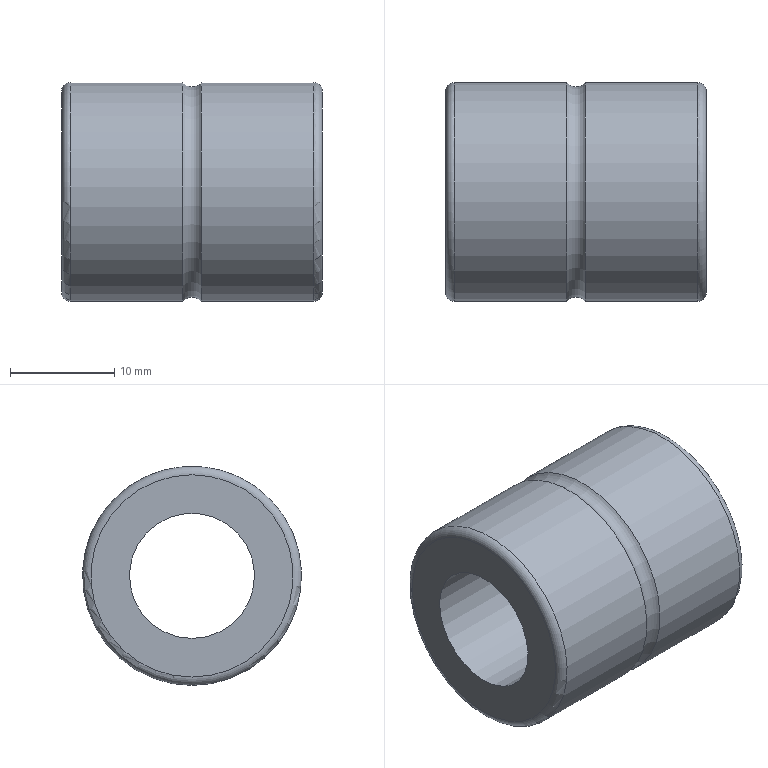Part | NX | features BREP 1 | 1 solid | 8 faces | box 25 x 21 x 21 mm | volume 5782 mm3 | torus 3 | cylinder 3 | plane 2 | commonest cylinder face diameters 21 x2 12 x1
STEP:
#1=CARTESIAN_POINT('',(0.,0.,-9.7));
#2=VERTEX_POINT('',#1);
#3=CARTESIAN_POINT('',(0.,0.,0.));
#4=DIRECTION('',(1.,0.,0.));
#5=DIRECTION('',(0.,0.,-1.));
#6=AXIS2_PLACEMENT_3D('',#3,#4,#5);
#7=CIRCLE('',#6,9.7);
#8=EDGE_CURVE('',#2,#2,#7,.T.);
#9=ORIENTED_EDGE('',*,*,#8,.F.);
#10=EDGE_LOOP('',(#9));
#11=FACE_BOUND('',#10,.T.);
#12=CARTESIAN_POINT('',(0.,0.,-6.));
#13=VERTEX_POINT('',#12);
#14=CARTESIAN_POINT('',(0.,0.,0.));
#15=DIRECTION('',(1.,0.,0.));
#16=DIRECTION('',(0.,0.,-1.));
#17=AXIS2_PLACEMENT_3D('',#14,#15,#16);
#18=CIRCLE('',#17,6.);
#19=EDGE_CURVE('',#13,#13,#18,.T.);
#20=ORIENTED_EDGE('',*,*,#19,.T.);
#21=EDGE_LOOP('',(#20));
#22=FACE_BOUND('',#21,.T.);
#23=CARTESIAN_POINT('',(0.,0.,0.));
#24=DIRECTION('',(1.,0.,0.));
#25=DIRECTION('',(0.,0.,1.));
#26=AXIS2_PLACEMENT_3D('',#23,#24,#25);
#27=PLANE('',#26);
#28=ADVANCED_FACE('',(#11,#22),#27,.F.);
#29=ORIENTED_EDGE('',*,*,#8,.T.);
#30=EDGE_LOOP('',(#29));
#31=FACE_BOUND('',#30,.T.);
#32=CARTESIAN_POINT('',(0.8,0.,-10.5));
#33=VERTEX_POINT('',#32);
#34=CARTESIAN_POINT('',(0.8,0.,0.));
#35=DIRECTION('',(1.,0.,0.));
#36=DIRECTION('',(0.,0.,-1.));
#37=AXIS2_PLACEMENT_3D('',#34,#35,#36);
#38=CIRCLE('',#37,10.5);
#39=EDGE_CURVE('',#33,#33,#38,.T.);
#40=ORIENTED_EDGE('',*,*,#39,.F.);
#41=EDGE_LOOP('',(#40));
#42=FACE_BOUND('',#41,.T.);
#43=CARTESIAN_POINT('',(0.8,0.,0.));
#44=DIRECTION('',(1.,0.,0.));
#45=DIRECTION('',(0.,0.,1.));
#46=AXIS2_PLACEMENT_3D('',#43,#44,#45);
#47=TOROIDAL_SURFACE('',#46,9.7,0.8);
#48=ADVANCED_FACE('',(#31,#42),#47,.T.);
#49=CARTESIAN_POINT('',(11.606,0.,-10.5));
#50=VERTEX_POINT('',#49);
#51=CARTESIAN_POINT('',(11.606,0.,0.));
#52=DIRECTION('',(1.,0.,0.));
#53=DIRECTION('',(0.,0.,-1.));
#54=AXIS2_PLACEMENT_3D('',#51,#52,#53);
#55=CIRCLE('',#54,10.5);
#56=EDGE_CURVE('',#50,#50,#55,.T.);
#57=ORIENTED_EDGE('',*,*,#56,.F.);
#58=EDGE_LOOP('',(#57));
#59=FACE_BOUND('',#58,.T.);
#60=ORIENTED_EDGE('',*,*,#39,.T.);
#61=EDGE_LOOP('',(#60));
#62=FACE_BOUND('',#61,.T.);
#63=CARTESIAN_POINT('',(25.,0.,0.));
#64=DIRECTION('',(1.,0.,0.));
#65=DIRECTION('',(0.,0.,1.));
#66=AXIS2_PLACEMENT_3D('',#63,#64,#65);
#67=CYLINDRICAL_SURFACE('',#66,10.5);
#68=ADVANCED_FACE('',(#59,#62),#67,.T.);
#69=CARTESIAN_POINT('',(13.394,0.,-10.5));
#70=VERTEX_POINT('',#69);
#71=CARTESIAN_POINT('',(13.394,0.,0.));
#72=DIRECTION('',(1.,0.,0.));
#73=DIRECTION('',(0.,0.,-1.));
#74=AXIS2_PLACEMENT_3D('',#71,#72,#73);
#75=CIRCLE('',#74,10.5);
#76=EDGE_CURVE('',#70,#70,#75,.T.);
#77=ORIENTED_EDGE('',*,*,#76,.F.);
#78=EDGE_LOOP('',(#77));
#79=FACE_BOUND('',#78,.T.);
#80=ORIENTED_EDGE('',*,*,#56,.T.);
#81=EDGE_LOOP('',(#80));
#82=FACE_BOUND('',#81,.T.);
#83=CARTESIAN_POINT('',(12.5,0.,0.));
#84=DIRECTION('',(1.,0.,0.));
#85=DIRECTION('',(0.,0.,1.));
#86=AXIS2_PLACEMENT_3D('',#83,#84,#85);
#87=TOROIDAL_SURFACE('',#86,11.3,1.2);
#88=ADVANCED_FACE('',(#79,#82),#87,.F.);
#89=CARTESIAN_POINT('',(24.2,0.,-10.5));
#90=VERTEX_POINT('',#89);
#91=CARTESIAN_POINT('',(24.2,0.,0.));
#92=DIRECTION('',(1.,0.,0.));
#93=DIRECTION('',(0.,0.,-1.));
#94=AXIS2_PLACEMENT_3D('',#91,#92,#93);
#95=CIRCLE('',#94,10.5);
#96=EDGE_CURVE('',#90,#90,#95,.T.);
#97=ORIENTED_EDGE('',*,*,#96,.F.);
#98=EDGE_LOOP('',(#97));
#99=FACE_BOUND('',#98,.T.);
#100=ORIENTED_EDGE('',*,*,#76,.T.);
#101=EDGE_LOOP('',(#100));
#102=FACE_BOUND('',#101,.T.);
#103=CARTESIAN_POINT('',(25.,0.,0.));
#104=DIRECTION('',(1.,0.,0.));
#105=DIRECTION('',(0.,0.,1.));
#106=AXIS2_PLACEMENT_3D('',#103,#104,#105);
#107=CYLINDRICAL_SURFACE('',#106,10.5);
#108=ADVANCED_FACE('',(#99,#102),#107,.T.);
#109=ORIENTED_EDGE('',*,*,#96,.T.);
#110=EDGE_LOOP('',(#109));
#111=FACE_BOUND('',#110,.T.);
#112=CARTESIAN_POINT('',(25.,0.,-9.7));
#113=VERTEX_POINT('',#112);
#114=CARTESIAN_POINT('',(25.,0.,0.));
#115=DIRECTION('',(1.,0.,0.));
#116=DIRECTION('',(0.,0.,-1.));
#117=AXIS2_PLACEMENT_3D('',#114,#115,#116);
#118=CIRCLE('',#117,9.7);
#119=EDGE_CURVE('',#113,#113,#118,.T.);
#120=ORIENTED_EDGE('',*,*,#119,.F.);
#121=EDGE_LOOP('',(#120));
#122=FACE_BOUND('',#121,.T.);
#123=CARTESIAN_POINT('',(24.2,0.,0.));
#124=DIRECTION('',(1.,0.,0.));
#125=DIRECTION('',(0.,0.,1.));
#126=AXIS2_PLACEMENT_3D('',#123,#124,#125);
#127=TOROIDAL_SURFACE('',#126,9.7,0.8);
#128=ADVANCED_FACE('',(#111,#122),#127,.T.);
#129=CARTESIAN_POINT('',(25.,0.,-6.));
#130=VERTEX_POINT('',#129);
#131=CARTESIAN_POINT('',(25.,0.,0.));
#132=DIRECTION('',(1.,0.,0.));
#133=DIRECTION('',(0.,0.,-1.));
#134=AXIS2_PLACEMENT_3D('',#131,#132,#133);
#135=CIRCLE('',#134,6.);
#136=EDGE_CURVE('',#130,#130,#135,.T.);
#137=ORIENTED_EDGE('',*,*,#136,.F.);
#138=EDGE_LOOP('',(#137));
#139=FACE_BOUND('',#138,.T.);
#140=ORIENTED_EDGE('',*,*,#119,.T.);
#141=EDGE_LOOP('',(#140));
#142=FACE_BOUND('',#141,.T.);
#143=CARTESIAN_POINT('',(25.,9.7,0.));
#144=DIRECTION('',(-1.,0.,0.));
#145=DIRECTION('',(0.,0.,-1.));
#146=AXIS2_PLACEMENT_3D('',#143,#144,#145);
#147=PLANE('',#146);
#148=ADVANCED_FACE('',(#139,#142),#147,.F.);
#149=ORIENTED_EDGE('',*,*,#136,.T.);
#150=EDGE_LOOP('',(#149));
#151=FACE_BOUND('',#150,.T.);
#152=ORIENTED_EDGE('',*,*,#19,.F.);
#153=EDGE_LOOP('',(#152));
#154=FACE_BOUND('',#153,.T.);
#155=CARTESIAN_POINT('',(25.,0.,0.));
#156=DIRECTION('',(1.,0.,0.));
#157=DIRECTION('',(0.,0.,1.));
#158=AXIS2_PLACEMENT_3D('',#155,#156,#157);
#159=CYLINDRICAL_SURFACE('',#158,6.);
#160=ADVANCED_FACE('',(#151,#154),#159,.F.);
#161=CLOSED_SHELL('',(#28,#48,#68,#88,#108,#128,#148,#160));
#162=MANIFOLD_SOLID_BREP('',#161);
#163=(LENGTH_UNIT()NAMED_UNIT(*)SI_UNIT(.MILLI.,.METRE.));
#164=UNCERTAINTY_MEASURE_WITH_UNIT(LENGTH_MEASURE(0.00001),#163,'','');
#165=(NAMED_UNIT(*)PLANE_ANGLE_UNIT()SI_UNIT($,.RADIAN.));
#166=(NAMED_UNIT(*)SI_UNIT($,.STERADIAN.)SOLID_ANGLE_UNIT());
#167=(GEOMETRIC_REPRESENTATION_CONTEXT(3)GLOBAL_UNCERTAINTY_ASSIGNED_CONTEXT((#164))GLOBAL_UNIT_ASSIGNED_CONTEXT((#163,#165,#166))REPRESENTATION_CONTEXT('',''));
#168=ADVANCED_BREP_SHAPE_REPRESENTATION('',(#162),#167);